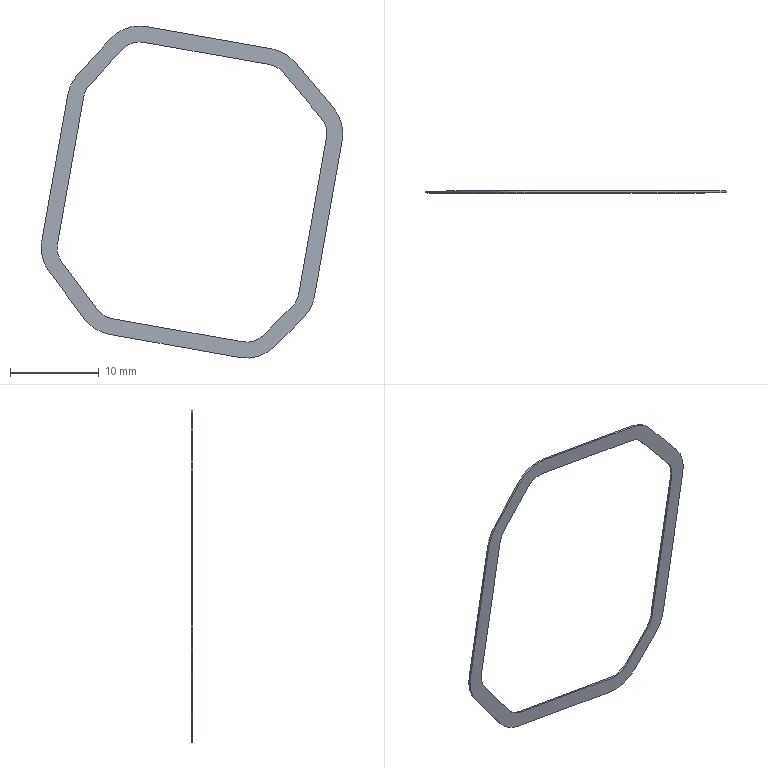Part | SolidWorks | features BaseBody 1 | 1 solid | 34 faces | box 34.044 x 0.2 x 37.494 mm | volume 39.583 mm3 | plane 18 | cylinder 16 | commonest cylinder face diameters 5.4 x8 9 x8
STEP:
#1=CARTESIAN_POINT('',(2064.15,-43.955,814.22));
#2=VERTEX_POINT('',#1);
#3=CARTESIAN_POINT('',(2064.15,-44.155,814.22));
#4=VERTEX_POINT('',#3);
#5=CARTESIAN_POINT('',(2064.15,-43.955,814.22));
#6=DIRECTION('',(0.,-1.,0.));
#7=VECTOR('',#6,1000.);
#8=LINE('',#5,#7);
#9=EDGE_CURVE('',#2,#4,#8,.T.);
#10=ORIENTED_EDGE('',*,*,#9,.T.);
#11=CARTESIAN_POINT('',(2049.484,-44.155,816.823));
#12=VERTEX_POINT('',#11);
#13=CARTESIAN_POINT('',(2049.484,-44.155,816.823));
#14=DIRECTION('',(0.9846,0.,-0.1747));
#15=VECTOR('',#14,1000.);
#16=LINE('',#13,#15);
#17=EDGE_CURVE('',#12,#4,#16,.T.);
#18=ORIENTED_EDGE('',*,*,#17,.F.);
#19=CARTESIAN_POINT('',(2049.484,-43.955,816.823));
#20=VERTEX_POINT('',#19);
#21=CARTESIAN_POINT('',(2049.484,-43.955,816.823));
#22=DIRECTION('',(0.,-1.,0.));
#23=VECTOR('',#22,1000.);
#24=LINE('',#21,#23);
#25=EDGE_CURVE('',#20,#12,#24,.T.);
#26=ORIENTED_EDGE('',*,*,#25,.F.);
#27=CARTESIAN_POINT('',(2049.484,-43.955,816.823));
#28=DIRECTION('',(0.9846,0.,-0.1747));
#29=VECTOR('',#28,1000.);
#30=LINE('',#27,#29);
#31=EDGE_CURVE('',#20,#2,#30,.T.);
#32=ORIENTED_EDGE('',*,*,#31,.T.);
#33=EDGE_LOOP('',(#10,#18,#26,#32));
#34=FACE_OUTER_BOUND('',#33,.T.);
#35=CARTESIAN_POINT('',(2049.484,-43.955,816.823));
#36=DIRECTION('',(-0.1747,0.,-0.9846));
#37=DIRECTION('',(-0.9846,0.,0.1747));
#38=AXIS2_PLACEMENT_3D('',#35,#36,#37);
#39=PLANE('',#38);
#40=ADVANCED_FACE('',(#34),#39,.T.);
#41=ORIENTED_EDGE('',*,*,#31,.F.);
#42=CARTESIAN_POINT('',(2046.674,-43.955,818.55));
#43=VERTEX_POINT('',#42);
#44=CARTESIAN_POINT('',(2050.27,-43.955,821.254));
#45=DIRECTION('',(0.,-1.,0.));
#46=DIRECTION('',(-0.7993,0.,-0.6009));
#47=AXIS2_PLACEMENT_3D('',#44,#45,#46);
#48=CIRCLE('',#47,4.5);
#49=EDGE_CURVE('',#43,#20,#48,.T.);
#50=ORIENTED_EDGE('',*,*,#49,.F.);
#51=CARTESIAN_POINT('',(2042.664,-43.955,823.882));
#52=VERTEX_POINT('',#51);
#53=CARTESIAN_POINT('',(2042.664,-43.955,823.882));
#54=DIRECTION('',(0.6009,0.,-0.7993));
#55=VECTOR('',#54,1000.);
#56=LINE('',#53,#55);
#57=EDGE_CURVE('',#52,#43,#56,.T.);
#58=ORIENTED_EDGE('',*,*,#57,.F.);
#59=CARTESIAN_POINT('',(2041.831,-43.955,827.373));
#60=VERTEX_POINT('',#59);
#61=CARTESIAN_POINT('',(2046.261,-43.955,826.586));
#62=DIRECTION('',(0.,-1.,0.));
#63=DIRECTION('',(-0.9846,0.,0.1747));
#64=AXIS2_PLACEMENT_3D('',#61,#62,#63);
#65=CIRCLE('',#64,4.5);
#66=EDGE_CURVE('',#60,#52,#65,.T.);
#67=ORIENTED_EDGE('',*,*,#66,.F.);
#68=CARTESIAN_POINT('',(2044.766,-43.955,843.914));
#69=VERTEX_POINT('',#68);
#70=CARTESIAN_POINT('',(2044.766,-43.955,843.914));
#71=DIRECTION('',(-0.1747,0.,-0.9846));
#72=VECTOR('',#71,1000.);
#73=LINE('',#70,#72);
#74=EDGE_CURVE('',#69,#60,#73,.T.);
#75=ORIENTED_EDGE('',*,*,#74,.F.);
#76=CARTESIAN_POINT('',(2045.883,-43.955,846.172));
#77=VERTEX_POINT('',#76);
#78=CARTESIAN_POINT('',(2049.197,-43.955,843.128));
#79=DIRECTION('',(0.,-1.,0.));
#80=DIRECTION('',(-0.7365,0.,0.6764));
#81=AXIS2_PLACEMENT_3D('',#78,#79,#80);
#82=CIRCLE('',#81,4.5);
#83=EDGE_CURVE('',#77,#69,#82,.T.);
#84=ORIENTED_EDGE('',*,*,#83,.F.);
#85=CARTESIAN_POINT('',(2049.572,-43.955,850.189));
#86=VERTEX_POINT('',#85);
#87=CARTESIAN_POINT('',(2049.572,-43.955,850.189));
#88=DIRECTION('',(-0.6764,0.,-0.7365));
#89=VECTOR('',#88,1000.);
#90=LINE('',#87,#89);
#91=EDGE_CURVE('',#86,#77,#90,.T.);
#92=ORIENTED_EDGE('',*,*,#91,.F.);
#93=CARTESIAN_POINT('',(2053.673,-43.955,851.576));
#94=VERTEX_POINT('',#93);
#95=CARTESIAN_POINT('',(2052.886,-43.955,847.145));
#96=DIRECTION('',(0.,-1.,0.));
#97=DIRECTION('',(0.1747,0.,0.9846));
#98=AXIS2_PLACEMENT_3D('',#95,#96,#97);
#99=CIRCLE('',#98,4.5);
#100=EDGE_CURVE('',#94,#86,#99,.T.);
#101=ORIENTED_EDGE('',*,*,#100,.F.);
#102=CARTESIAN_POINT('',(2067.797,-43.955,849.069));
#103=VERTEX_POINT('',#102);
#104=CARTESIAN_POINT('',(2067.797,-43.955,849.069));
#105=DIRECTION('',(-0.9846,0.,0.1747));
#106=VECTOR('',#105,1000.);
#107=LINE('',#104,#106);
#108=EDGE_CURVE('',#103,#94,#107,.T.);
#109=ORIENTED_EDGE('',*,*,#108,.F.);
#110=CARTESIAN_POINT('',(2070.461,-43.955,847.527));
#111=VERTEX_POINT('',#110);
#112=CARTESIAN_POINT('',(2067.011,-43.955,844.638));
#113=DIRECTION('',(0.,-1.,0.));
#114=DIRECTION('',(0.7668,0.,0.6419));
#115=AXIS2_PLACEMENT_3D('',#112,#113,#114);
#116=CIRCLE('',#115,4.5);
#117=EDGE_CURVE('',#111,#103,#116,.T.);
#118=ORIENTED_EDGE('',*,*,#117,.F.);
#119=CARTESIAN_POINT('',(2074.755,-43.955,842.398));
#120=VERTEX_POINT('',#119);
#121=CARTESIAN_POINT('',(2074.755,-43.955,842.398));
#122=DIRECTION('',(-0.6419,0.,0.7668));
#123=VECTOR('',#122,1000.);
#124=LINE('',#121,#123);
#125=EDGE_CURVE('',#120,#111,#124,.T.);
#126=ORIENTED_EDGE('',*,*,#125,.F.);
#127=CARTESIAN_POINT('',(2075.736,-43.955,838.723));
#128=VERTEX_POINT('',#127);
#129=CARTESIAN_POINT('',(2071.305,-43.955,839.509));
#130=DIRECTION('',(0.,-1.,0.));
#131=DIRECTION('',(0.9846,0.,-0.1747));
#132=AXIS2_PLACEMENT_3D('',#129,#130,#131);
#133=CIRCLE('',#132,4.5);
#134=EDGE_CURVE('',#128,#120,#133,.T.);
#135=ORIENTED_EDGE('',*,*,#134,.F.);
#136=CARTESIAN_POINT('',(2072.608,-43.955,821.098));
#137=VERTEX_POINT('',#136);
#138=CARTESIAN_POINT('',(2072.608,-43.955,821.098));
#139=DIRECTION('',(0.1747,0.,0.9846));
#140=VECTOR('',#139,1000.);
#141=LINE('',#138,#140);
#142=EDGE_CURVE('',#137,#128,#141,.T.);
#143=ORIENTED_EDGE('',*,*,#142,.F.);
#144=CARTESIAN_POINT('',(2071.355,-43.955,818.699));
#145=VERTEX_POINT('',#144);
#146=CARTESIAN_POINT('',(2068.177,-43.955,821.884));
#147=DIRECTION('',(0.,-1.,0.));
#148=DIRECTION('',(0.7063,0.,-0.7079));
#149=AXIS2_PLACEMENT_3D('',#146,#147,#148);
#150=CIRCLE('',#149,4.5);
#151=EDGE_CURVE('',#145,#137,#150,.T.);
#152=ORIENTED_EDGE('',*,*,#151,.F.);
#153=CARTESIAN_POINT('',(2068.115,-43.955,815.465));
#154=VERTEX_POINT('',#153);
#155=CARTESIAN_POINT('',(2068.115,-43.955,815.465));
#156=DIRECTION('',(0.7079,0.,0.7063));
#157=VECTOR('',#156,1000.);
#158=LINE('',#155,#157);
#159=EDGE_CURVE('',#154,#145,#158,.T.);
#160=ORIENTED_EDGE('',*,*,#159,.F.);
#161=CARTESIAN_POINT('',(2064.936,-43.955,818.651));
#162=DIRECTION('',(0.,-1.,0.));
#163=DIRECTION('',(-0.1747,0.,-0.9846));
#164=AXIS2_PLACEMENT_3D('',#161,#162,#163);
#165=CIRCLE('',#164,4.5);
#166=EDGE_CURVE('',#2,#154,#165,.T.);
#167=ORIENTED_EDGE('',*,*,#166,.F.);
#168=EDGE_LOOP('',(#41,#50,#58,#67,#75,#84,#92,#101,#109,#118,#126,#135,#143,#152,#160,#167));
#169=FACE_OUTER_BOUND('',#168,.T.);
#170=CARTESIAN_POINT('',(2066.843,-43.955,816.74));
#171=VERTEX_POINT('',#170);
#172=CARTESIAN_POINT('',(2064.464,-43.955,815.992));
#173=VERTEX_POINT('',#172);
#174=CARTESIAN_POINT('',(2064.936,-43.955,818.651));
#175=DIRECTION('',(0.,1.,0.));
#176=DIRECTION('',(0.7063,0.,-0.7079));
#177=AXIS2_PLACEMENT_3D('',#174,#175,#176);
#178=CIRCLE('',#177,2.7);
#179=EDGE_CURVE('',#171,#173,#178,.T.);
#180=ORIENTED_EDGE('',*,*,#179,.F.);
#181=CARTESIAN_POINT('',(2070.084,-43.955,819.973));
#182=VERTEX_POINT('',#181);
#183=CARTESIAN_POINT('',(2070.084,-43.955,819.973));
#184=DIRECTION('',(-0.7079,0.,-0.7063));
#185=VECTOR('',#184,1000.);
#186=LINE('',#183,#185);
#187=EDGE_CURVE('',#182,#171,#186,.T.);
#188=ORIENTED_EDGE('',*,*,#187,.F.);
#189=CARTESIAN_POINT('',(2070.835,-43.955,821.413));
#190=VERTEX_POINT('',#189);
#191=CARTESIAN_POINT('',(2068.177,-43.955,821.884));
#192=DIRECTION('',(0.,1.,0.));
#193=DIRECTION('',(0.9846,0.,-0.1747));
#194=AXIS2_PLACEMENT_3D('',#191,#192,#193);
#195=CIRCLE('',#194,2.7);
#196=EDGE_CURVE('',#190,#182,#195,.T.);
#197=ORIENTED_EDGE('',*,*,#196,.F.);
#198=CARTESIAN_POINT('',(2073.963,-43.955,839.037));
#199=VERTEX_POINT('',#198);
#200=CARTESIAN_POINT('',(2073.963,-43.955,839.037));
#201=DIRECTION('',(-0.1747,0.,-0.9846));
#202=VECTOR('',#201,1000.);
#203=LINE('',#200,#202);
#204=EDGE_CURVE('',#199,#190,#203,.T.);
#205=ORIENTED_EDGE('',*,*,#204,.F.);
#206=CARTESIAN_POINT('',(2073.375,-43.955,841.242));
#207=VERTEX_POINT('',#206);
#208=CARTESIAN_POINT('',(2071.305,-43.955,839.509));
#209=DIRECTION('',(0.,1.,0.));
#210=DIRECTION('',(0.7668,0.,0.6419));
#211=AXIS2_PLACEMENT_3D('',#208,#209,#210);
#212=CIRCLE('',#211,2.7);
#213=EDGE_CURVE('',#207,#199,#212,.T.);
#214=ORIENTED_EDGE('',*,*,#213,.F.);
#215=CARTESIAN_POINT('',(2069.081,-43.955,846.371));
#216=VERTEX_POINT('',#215);
#217=CARTESIAN_POINT('',(2069.081,-43.955,846.371));
#218=DIRECTION('',(0.6419,0.,-0.7668));
#219=VECTOR('',#218,1000.);
#220=LINE('',#217,#219);
#221=EDGE_CURVE('',#216,#207,#220,.T.);
#222=ORIENTED_EDGE('',*,*,#221,.F.);
#223=CARTESIAN_POINT('',(2067.482,-43.955,847.297));
#224=VERTEX_POINT('',#223);
#225=CARTESIAN_POINT('',(2067.011,-43.955,844.638));
#226=DIRECTION('',(0.,1.,0.));
#227=DIRECTION('',(0.1747,0.,0.9846));
#228=AXIS2_PLACEMENT_3D('',#225,#226,#227);
#229=CIRCLE('',#228,2.7);
#230=EDGE_CURVE('',#224,#216,#229,.T.);
#231=ORIENTED_EDGE('',*,*,#230,.F.);
#232=CARTESIAN_POINT('',(2053.358,-43.955,849.803));
#233=VERTEX_POINT('',#232);
#234=CARTESIAN_POINT('',(2053.358,-43.955,849.803));
#235=DIRECTION('',(0.9846,0.,-0.1747));
#236=VECTOR('',#235,1000.);
#237=LINE('',#234,#236);
#238=EDGE_CURVE('',#233,#224,#237,.T.);
#239=ORIENTED_EDGE('',*,*,#238,.F.);
#240=CARTESIAN_POINT('',(2050.898,-43.955,848.971));
#241=VERTEX_POINT('',#240);
#242=CARTESIAN_POINT('',(2052.886,-43.955,847.145));
#243=DIRECTION('',(0.,1.,0.));
#244=DIRECTION('',(-0.7365,0.,0.6764));
#245=AXIS2_PLACEMENT_3D('',#242,#243,#244);
#246=CIRCLE('',#245,2.7);
#247=EDGE_CURVE('',#241,#233,#246,.T.);
#248=ORIENTED_EDGE('',*,*,#247,.F.);
#249=CARTESIAN_POINT('',(2047.209,-43.955,844.954));
#250=VERTEX_POINT('',#249);
#251=CARTESIAN_POINT('',(2047.209,-43.955,844.954));
#252=DIRECTION('',(0.6764,0.,0.7365));
#253=VECTOR('',#252,1000.);
#254=LINE('',#251,#253);
#255=EDGE_CURVE('',#250,#241,#254,.T.);
#256=ORIENTED_EDGE('',*,*,#255,.F.);
#257=CARTESIAN_POINT('',(2046.539,-43.955,843.6));
#258=VERTEX_POINT('',#257);
#259=CARTESIAN_POINT('',(2049.197,-43.955,843.128));
#260=DIRECTION('',(0.,1.,0.));
#261=DIRECTION('',(-0.9846,0.,0.1747));
#262=AXIS2_PLACEMENT_3D('',#259,#260,#261);
#263=CIRCLE('',#262,2.7);
#264=EDGE_CURVE('',#258,#250,#263,.T.);
#265=ORIENTED_EDGE('',*,*,#264,.F.);
#266=CARTESIAN_POINT('',(2043.603,-43.955,827.058));
#267=VERTEX_POINT('',#266);
#268=CARTESIAN_POINT('',(2043.603,-43.955,827.058));
#269=DIRECTION('',(0.1747,0.,0.9846));
#270=VECTOR('',#269,1000.);
#271=LINE('',#268,#270);
#272=EDGE_CURVE('',#267,#258,#271,.T.);
#273=ORIENTED_EDGE('',*,*,#272,.F.);
#274=CARTESIAN_POINT('',(2044.103,-43.955,824.964));
#275=VERTEX_POINT('',#274);
#276=CARTESIAN_POINT('',(2046.261,-43.955,826.586));
#277=DIRECTION('',(0.,1.,0.));
#278=DIRECTION('',(-0.7993,0.,-0.6009));
#279=AXIS2_PLACEMENT_3D('',#276,#277,#278);
#280=CIRCLE('',#279,2.7);
#281=EDGE_CURVE('',#275,#267,#280,.T.);
#282=ORIENTED_EDGE('',*,*,#281,.F.);
#283=CARTESIAN_POINT('',(2048.112,-43.955,819.631));
#284=VERTEX_POINT('',#283);
#285=CARTESIAN_POINT('',(2048.112,-43.955,819.631));
#286=DIRECTION('',(-0.6009,0.,0.7993));
#287=VECTOR('',#286,1000.);
#288=LINE('',#285,#287);
#289=EDGE_CURVE('',#284,#275,#288,.T.);
#290=ORIENTED_EDGE('',*,*,#289,.F.);
#291=CARTESIAN_POINT('',(2049.799,-43.955,818.595));
#292=VERTEX_POINT('',#291);
#293=CARTESIAN_POINT('',(2050.27,-43.955,821.254));
#294=DIRECTION('',(0.,1.,0.));
#295=DIRECTION('',(-0.1747,0.,-0.9846));
#296=AXIS2_PLACEMENT_3D('',#293,#294,#295);
#297=CIRCLE('',#296,2.7);
#298=EDGE_CURVE('',#292,#284,#297,.T.);
#299=ORIENTED_EDGE('',*,*,#298,.F.);
#300=CARTESIAN_POINT('',(2064.464,-43.955,815.992));
#301=DIRECTION('',(-0.9846,0.,0.1747));
#302=VECTOR('',#301,1000.);
#303=LINE('',#300,#302);
#304=EDGE_CURVE('',#173,#292,#303,.T.);
#305=ORIENTED_EDGE('',*,*,#304,.F.);
#306=EDGE_LOOP('',(#180,#188,#197,#205,#214,#222,#231,#239,#248,#256,#265,#273,#282,#290,#299,#305));
#307=FACE_BOUND('',#306,.T.);
#308=CARTESIAN_POINT('',(2032.4,-43.955,838.898));
#309=DIRECTION('',(0.,-1.,0.));
#310=DIRECTION('',(-0.9846,0.,0.1747));
#311=AXIS2_PLACEMENT_3D('',#308,#309,#310);
#312=PLANE('',#311);
#313=ADVANCED_FACE('',(#169,#307),#312,.F.);
#314=CARTESIAN_POINT('',(2068.115,-44.155,815.465));
#315=VERTEX_POINT('',#314);
#316=CARTESIAN_POINT('',(2068.115,-43.955,815.465));
#317=DIRECTION('',(0.,-1.,0.));
#318=VECTOR('',#317,1000.);
#319=LINE('',#316,#318);
#320=EDGE_CURVE('',#154,#315,#319,.T.);
#321=ORIENTED_EDGE('',*,*,#320,.T.);
#322=CARTESIAN_POINT('',(2064.936,-44.155,818.651));
#323=DIRECTION('',(0.,-1.,0.));
#324=DIRECTION('',(-0.1747,0.,-0.9846));
#325=AXIS2_PLACEMENT_3D('',#322,#323,#324);
#326=CIRCLE('',#325,4.5);
#327=EDGE_CURVE('',#4,#315,#326,.T.);
#328=ORIENTED_EDGE('',*,*,#327,.F.);
#329=ORIENTED_EDGE('',*,*,#9,.F.);
#330=ORIENTED_EDGE('',*,*,#166,.T.);
#331=EDGE_LOOP('',(#321,#328,#329,#330));
#332=FACE_OUTER_BOUND('',#331,.T.);
#333=CARTESIAN_POINT('',(2064.936,-43.955,818.651));
#334=DIRECTION('',(0.,-1.,0.));
#335=DIRECTION('',(-0.9846,0.,0.1747));
#336=AXIS2_PLACEMENT_3D('',#333,#334,#335);
#337=CYLINDRICAL_SURFACE('',#336,4.5);
#338=ADVANCED_FACE('',(#332),#337,.T.);
#339=CARTESIAN_POINT('',(2071.355,-44.155,818.699));
#340=VERTEX_POINT('',#339);
#341=CARTESIAN_POINT('',(2068.115,-44.155,815.465));
#342=DIRECTION('',(0.7079,0.,0.7063));
#343=VECTOR('',#342,1000.);
#344=LINE('',#341,#343);
#345=EDGE_CURVE('',#315,#340,#344,.T.);
#346=ORIENTED_EDGE('',*,*,#345,.T.);
#347=CARTESIAN_POINT('',(2072.608,-44.155,821.098));
#348=VERTEX_POINT('',#347);
#349=CARTESIAN_POINT('',(2068.177,-44.155,821.884));
#350=DIRECTION('',(0.,-1.,0.));
#351=DIRECTION('',(0.7063,0.,-0.7079));
#352=AXIS2_PLACEMENT_3D('',#349,#350,#351);
#353=CIRCLE('',#352,4.5);
#354=EDGE_CURVE('',#340,#348,#353,.T.);
#355=ORIENTED_EDGE('',*,*,#354,.T.);
#356=CARTESIAN_POINT('',(2075.736,-44.155,838.723));
#357=VERTEX_POINT('',#356);
#358=CARTESIAN_POINT('',(2072.608,-44.155,821.098));
#359=DIRECTION('',(0.1747,0.,0.9846));
#360=VECTOR('',#359,1000.);
#361=LINE('',#358,#360);
#362=EDGE_CURVE('',#348,#357,#361,.T.);
#363=ORIENTED_EDGE('',*,*,#362,.T.);
#364=CARTESIAN_POINT('',(2074.755,-44.155,842.398));
#365=VERTEX_POINT('',#364);
#366=CARTESIAN_POINT('',(2071.305,-44.155,839.509));
#367=DIRECTION('',(0.,-1.,0.));
#368=DIRECTION('',(0.9846,0.,-0.1747));
#369=AXIS2_PLACEMENT_3D('',#366,#367,#368);
#370=CIRCLE('',#369,4.5);
#371=EDGE_CURVE('',#357,#365,#370,.T.);
#372=ORIENTED_EDGE('',*,*,#371,.T.);
#373=CARTESIAN_POINT('',(2070.461,-44.155,847.527));
#374=VERTEX_POINT('',#373);
#375=CARTESIAN_POINT('',(2074.755,-44.155,842.398));
#376=DIRECTION('',(-0.6419,0.,0.7668));
#377=VECTOR('',#376,1000.);
#378=LINE('',#375,#377);
#379=EDGE_CURVE('',#365,#374,#378,.T.);
#380=ORIENTED_EDGE('',*,*,#379,.T.);
#381=CARTESIAN_POINT('',(2067.797,-44.155,849.069));
#382=VERTEX_POINT('',#381);
#383=CARTESIAN_POINT('',(2067.011,-44.155,844.638));
#384=DIRECTION('',(0.,-1.,0.));
#385=DIRECTION('',(0.7668,0.,0.6419));
#386=AXIS2_PLACEMENT_3D('',#383,#384,#385);
#387=CIRCLE('',#386,4.5);
#388=EDGE_CURVE('',#374,#382,#387,.T.);
#389=ORIENTED_EDGE('',*,*,#388,.T.);
#390=CARTESIAN_POINT('',(2053.673,-44.155,851.576));
#391=VERTEX_POINT('',#390);
#392=CARTESIAN_POINT('',(2067.797,-44.155,849.069));
#393=DIRECTION('',(-0.9846,0.,0.1747));
#394=VECTOR('',#393,1000.);
#395=LINE('',#392,#394);
#396=EDGE_CURVE('',#382,#391,#395,.T.);
#397=ORIENTED_EDGE('',*,*,#396,.T.);
#398=CARTESIAN_POINT('',(2049.572,-44.155,850.189));
#399=VERTEX_POINT('',#398);
#400=CARTESIAN_POINT('',(2052.886,-44.155,847.145));
#401=DIRECTION('',(0.,-1.,0.));
#402=DIRECTION('',(0.1747,0.,0.9846));
#403=AXIS2_PLACEMENT_3D('',#400,#401,#402);
#404=CIRCLE('',#403,4.5);
#405=EDGE_CURVE('',#391,#399,#404,.T.);
#406=ORIENTED_EDGE('',*,*,#405,.T.);
#407=CARTESIAN_POINT('',(2045.883,-44.155,846.172));
#408=VERTEX_POINT('',#407);
#409=CARTESIAN_POINT('',(2049.572,-44.155,850.189));
#410=DIRECTION('',(-0.6764,0.,-0.7365));
#411=VECTOR('',#410,1000.);
#412=LINE('',#409,#411);
#413=EDGE_CURVE('',#399,#408,#412,.T.);
#414=ORIENTED_EDGE('',*,*,#413,.T.);
#415=CARTESIAN_POINT('',(2044.766,-44.155,843.914));
#416=VERTEX_POINT('',#415);
#417=CARTESIAN_POINT('',(2049.197,-44.155,843.128));
#418=DIRECTION('',(0.,-1.,0.));
#419=DIRECTION('',(-0.7365,0.,0.6764));
#420=AXIS2_PLACEMENT_3D('',#417,#418,#419);
#421=CIRCLE('',#420,4.5);
#422=EDGE_CURVE('',#408,#416,#421,.T.);
#423=ORIENTED_EDGE('',*,*,#422,.T.);
#424=CARTESIAN_POINT('',(2041.831,-44.155,827.373));
#425=VERTEX_POINT('',#424);
#426=CARTESIAN_POINT('',(2044.766,-44.155,843.914));
#427=DIRECTION('',(-0.1747,0.,-0.9846));
#428=VECTOR('',#427,1000.);
#429=LINE('',#426,#428);
#430=EDGE_CURVE('',#416,#425,#429,.T.);
#431=ORIENTED_EDGE('',*,*,#430,.T.);
#432=CARTESIAN_POINT('',(2042.664,-44.155,823.882));
#433=VERTEX_POINT('',#432);
#434=CARTESIAN_POINT('',(2046.261,-44.155,826.586));
#435=DIRECTION('',(0.,-1.,0.));
#436=DIRECTION('',(-0.9846,0.,0.1747));
#437=AXIS2_PLACEMENT_3D('',#434,#435,#436);
#438=CIRCLE('',#437,4.5);
#439=EDGE_CURVE('',#425,#433,#438,.T.);
#440=ORIENTED_EDGE('',*,*,#439,.T.);
#441=CARTESIAN_POINT('',(2046.674,-44.155,818.55));
#442=VERTEX_POINT('',#441);
#443=CARTESIAN_POINT('',(2042.664,-44.155,823.882));
#444=DIRECTION('',(0.6009,0.,-0.7993));
#445=VECTOR('',#444,1000.);
#446=LINE('',#443,#445);
#447=EDGE_CURVE('',#433,#442,#446,.T.);
#448=ORIENTED_EDGE('',*,*,#447,.T.);
#449=CARTESIAN_POINT('',(2050.27,-44.155,821.254));
#450=DIRECTION('',(0.,-1.,0.));
#451=DIRECTION('',(-0.7993,0.,-0.6009));
#452=AXIS2_PLACEMENT_3D('',#449,#450,#451);
#453=CIRCLE('',#452,4.5);
#454=EDGE_CURVE('',#442,#12,#453,.T.);
#455=ORIENTED_EDGE('',*,*,#454,.T.);
#456=ORIENTED_EDGE('',*,*,#17,.T.);
#457=ORIENTED_EDGE('',*,*,#327,.T.);
#458=EDGE_LOOP('',(#346,#355,#363,#372,#380,#389,#397,#406,#414,#423,#431,#440,#448,#455,#456,#457));
#459=FACE_OUTER_BOUND('',#458,.T.);
#460=CARTESIAN_POINT('',(2049.799,-44.155,818.595));
#461=VERTEX_POINT('',#460);
#462=CARTESIAN_POINT('',(2048.112,-44.155,819.631));
#463=VERTEX_POINT('',#462);
#464=CARTESIAN_POINT('',(2050.27,-44.155,821.254));
#465=DIRECTION('',(0.,1.,0.));
#466=DIRECTION('',(-0.1747,0.,-0.9846));
#467=AXIS2_PLACEMENT_3D('',#464,#465,#466);
#468=CIRCLE('',#467,2.7);
#469=EDGE_CURVE('',#461,#463,#468,.T.);
#470=ORIENTED_EDGE('',*,*,#469,.T.);
#471=CARTESIAN_POINT('',(2044.103,-44.155,824.964));
#472=VERTEX_POINT('',#471);
#473=CARTESIAN_POINT('',(2048.112,-44.155,819.631));
#474=DIRECTION('',(-0.6009,0.,0.7993));
#475=VECTOR('',#474,1000.);
#476=LINE('',#473,#475);
#477=EDGE_CURVE('',#463,#472,#476,.T.);
#478=ORIENTED_EDGE('',*,*,#477,.T.);
#479=CARTESIAN_POINT('',(2043.603,-44.155,827.058));
#480=VERTEX_POINT('',#479);
#481=CARTESIAN_POINT('',(2046.261,-44.155,826.586));
#482=DIRECTION('',(0.,1.,0.));
#483=DIRECTION('',(-0.7993,0.,-0.6009));
#484=AXIS2_PLACEMENT_3D('',#481,#482,#483);
#485=CIRCLE('',#484,2.7);
#486=EDGE_CURVE('',#472,#480,#485,.T.);
#487=ORIENTED_EDGE('',*,*,#486,.T.);
#488=CARTESIAN_POINT('',(2046.539,-44.155,843.6));
#489=VERTEX_POINT('',#488);
#490=CARTESIAN_POINT('',(2043.603,-44.155,827.058));
#491=DIRECTION('',(0.1747,0.,0.9846));
#492=VECTOR('',#491,1000.);
#493=LINE('',#490,#492);
#494=EDGE_CURVE('',#480,#489,#493,.T.);
#495=ORIENTED_EDGE('',*,*,#494,.T.);
#496=CARTESIAN_POINT('',(2047.209,-44.155,844.954));
#497=VERTEX_POINT('',#496);
#498=CARTESIAN_POINT('',(2049.197,-44.155,843.128));
#499=DIRECTION('',(0.,1.,0.));
#500=DIRECTION('',(-0.9846,0.,0.1747));
#501=AXIS2_PLACEMENT_3D('',#498,#499,#500);
#502=CIRCLE('',#501,2.7);
#503=EDGE_CURVE('',#489,#497,#502,.T.);
#504=ORIENTED_EDGE('',*,*,#503,.T.);
#505=CARTESIAN_POINT('',(2050.898,-44.155,848.971));
#506=VERTEX_POINT('',#505);
#507=CARTESIAN_POINT('',(2047.209,-44.155,844.954));
#508=DIRECTION('',(0.6764,0.,0.7365));
#509=VECTOR('',#508,1000.);
#510=LINE('',#507,#509);
#511=EDGE_CURVE('',#497,#506,#510,.T.);
#512=ORIENTED_EDGE('',*,*,#511,.T.);
#513=CARTESIAN_POINT('',(2053.358,-44.155,849.803));
#514=VERTEX_POINT('',#513);
#515=CARTESIAN_POINT('',(2052.886,-44.155,847.145));
#516=DIRECTION('',(0.,1.,0.));
#517=DIRECTION('',(-0.7365,0.,0.6764));
#518=AXIS2_PLACEMENT_3D('',#515,#516,#517);
#519=CIRCLE('',#518,2.7);
#520=EDGE_CURVE('',#506,#514,#519,.T.);
#521=ORIENTED_EDGE('',*,*,#520,.T.);
#522=CARTESIAN_POINT('',(2067.482,-44.155,847.297));
#523=VERTEX_POINT('',#522);
#524=CARTESIAN_POINT('',(2053.358,-44.155,849.803));
#525=DIRECTION('',(0.9846,0.,-0.1747));
#526=VECTOR('',#525,1000.);
#527=LINE('',#524,#526);
#528=EDGE_CURVE('',#514,#523,#527,.T.);
#529=ORIENTED_EDGE('',*,*,#528,.T.);
#530=CARTESIAN_POINT('',(2069.081,-44.155,846.371));
#531=VERTEX_POINT('',#530);
#532=CARTESIAN_POINT('',(2067.011,-44.155,844.638));
#533=DIRECTION('',(0.,1.,0.));
#534=DIRECTION('',(0.1747,0.,0.9846));
#535=AXIS2_PLACEMENT_3D('',#532,#533,#534);
#536=CIRCLE('',#535,2.7);
#537=EDGE_CURVE('',#523,#531,#536,.T.);
#538=ORIENTED_EDGE('',*,*,#537,.T.);
#539=CARTESIAN_POINT('',(2073.375,-44.155,841.242));
#540=VERTEX_POINT('',#539);
#541=CARTESIAN_POINT('',(2069.081,-44.155,846.371));
#542=DIRECTION('',(0.6419,0.,-0.7668));
#543=VECTOR('',#542,1000.);
#544=LINE('',#541,#543);
#545=EDGE_CURVE('',#531,#540,#544,.T.);
#546=ORIENTED_EDGE('',*,*,#545,.T.);
#547=CARTESIAN_POINT('',(2073.963,-44.155,839.037));
#548=VERTEX_POINT('',#547);
#549=CARTESIAN_POINT('',(2071.305,-44.155,839.509));
#550=DIRECTION('',(0.,1.,0.));
#551=DIRECTION('',(0.7668,0.,0.6419));
#552=AXIS2_PLACEMENT_3D('',#549,#550,#551);
#553=CIRCLE('',#552,2.7);
#554=EDGE_CURVE('',#540,#548,#553,.T.);
#555=ORIENTED_EDGE('',*,*,#554,.T.);
#556=CARTESIAN_POINT('',(2070.835,-44.155,821.413));
#557=VERTEX_POINT('',#556);
#558=CARTESIAN_POINT('',(2073.963,-44.155,839.037));
#559=DIRECTION('',(-0.1747,0.,-0.9846));
#560=VECTOR('',#559,1000.);
#561=LINE('',#558,#560);
#562=EDGE_CURVE('',#548,#557,#561,.T.);
#563=ORIENTED_EDGE('',*,*,#562,.T.);
#564=CARTESIAN_POINT('',(2070.084,-44.155,819.973));
#565=VERTEX_POINT('',#564);
#566=CARTESIAN_POINT('',(2068.177,-44.155,821.884));
#567=DIRECTION('',(0.,1.,0.));
#568=DIRECTION('',(0.9846,0.,-0.1747));
#569=AXIS2_PLACEMENT_3D('',#566,#567,#568);
#570=CIRCLE('',#569,2.7);
#571=EDGE_CURVE('',#557,#565,#570,.T.);
#572=ORIENTED_EDGE('',*,*,#571,.T.);
#573=CARTESIAN_POINT('',(2066.843,-44.155,816.74));
#574=VERTEX_POINT('',#573);
#575=CARTESIAN_POINT('',(2070.084,-44.155,819.973));
#576=DIRECTION('',(-0.7079,0.,-0.7063));
#577=VECTOR('',#576,1000.);
#578=LINE('',#575,#577);
#579=EDGE_CURVE('',#565,#574,#578,.T.);
#580=ORIENTED_EDGE('',*,*,#579,.T.);
#581=CARTESIAN_POINT('',(2064.464,-44.155,815.992));
#582=VERTEX_POINT('',#581);
#583=CARTESIAN_POINT('',(2064.936,-44.155,818.651));
#584=DIRECTION('',(0.,1.,0.));
#585=DIRECTION('',(0.7063,0.,-0.7079));
#586=AXIS2_PLACEMENT_3D('',#583,#584,#585);
#587=CIRCLE('',#586,2.7);
#588=EDGE_CURVE('',#574,#582,#587,.T.);
#589=ORIENTED_EDGE('',*,*,#588,.T.);
#590=CARTESIAN_POINT('',(2064.464,-44.155,815.992));
#591=DIRECTION('',(-0.9846,0.,0.1747));
#592=VECTOR('',#591,1000.);
#593=LINE('',#590,#592);
#594=EDGE_CURVE('',#582,#461,#593,.T.);
#595=ORIENTED_EDGE('',*,*,#594,.T.);
#596=EDGE_LOOP('',(#470,#478,#487,#495,#504,#512,#521,#529,#538,#546,#555,#563,#572,#580,#589,#595));
#597=FACE_BOUND('',#596,.T.);
#598=CARTESIAN_POINT('',(2032.4,-44.155,838.898));
#599=DIRECTION('',(0.,-1.,0.));
#600=DIRECTION('',(-0.9846,0.,0.1747));
#601=AXIS2_PLACEMENT_3D('',#598,#599,#600);
#602=PLANE('',#601);
#603=ADVANCED_FACE('',(#459,#597),#602,.T.);
#604=ORIENTED_EDGE('',*,*,#25,.T.);
#605=ORIENTED_EDGE('',*,*,#454,.F.);
#606=CARTESIAN_POINT('',(2046.674,-43.955,818.55));
#607=DIRECTION('',(0.,-1.,0.));
#608=VECTOR('',#607,1000.);
#609=LINE('',#606,#608);
#610=EDGE_CURVE('',#43,#442,#609,.T.);
#611=ORIENTED_EDGE('',*,*,#610,.F.);
#612=ORIENTED_EDGE('',*,*,#49,.T.);
#613=EDGE_LOOP('',(#604,#605,#611,#612));
#614=FACE_OUTER_BOUND('',#613,.T.);
#615=CARTESIAN_POINT('',(2050.27,-43.955,821.254));
#616=DIRECTION('',(0.,-1.,0.));
#617=DIRECTION('',(-0.9846,0.,0.1747));
#618=AXIS2_PLACEMENT_3D('',#615,#616,#617);
#619=CYLINDRICAL_SURFACE('',#618,4.5);
#620=ADVANCED_FACE('',(#614),#619,.T.);
#621=ORIENTED_EDGE('',*,*,#610,.T.);
#622=ORIENTED_EDGE('',*,*,#447,.F.);
#623=CARTESIAN_POINT('',(2042.664,-43.955,823.882));
#624=DIRECTION('',(0.,-1.,0.));
#625=VECTOR('',#624,1000.);
#626=LINE('',#623,#625);
#627=EDGE_CURVE('',#52,#433,#626,.T.);
#628=ORIENTED_EDGE('',*,*,#627,.F.);
#629=ORIENTED_EDGE('',*,*,#57,.T.);
#630=EDGE_LOOP('',(#621,#622,#628,#629));
#631=FACE_OUTER_BOUND('',#630,.T.);
#632=CARTESIAN_POINT('',(2042.664,-43.955,823.882));
#633=DIRECTION('',(-0.7993,0.,-0.6009));
#634=DIRECTION('',(-0.6009,0.,0.7993));
#635=AXIS2_PLACEMENT_3D('',#632,#633,#634);
#636=PLANE('',#635);
#637=ADVANCED_FACE('',(#631),#636,.T.);
#638=ORIENTED_EDGE('',*,*,#627,.T.);
#639=ORIENTED_EDGE('',*,*,#439,.F.);
#640=CARTESIAN_POINT('',(2041.831,-43.955,827.373));
#641=DIRECTION('',(0.,-1.,0.));
#642=VECTOR('',#641,1000.);
#643=LINE('',#640,#642);
#644=EDGE_CURVE('',#60,#425,#643,.T.);
#645=ORIENTED_EDGE('',*,*,#644,.F.);
#646=ORIENTED_EDGE('',*,*,#66,.T.);
#647=EDGE_LOOP('',(#638,#639,#645,#646));
#648=FACE_OUTER_BOUND('',#647,.T.);
#649=CARTESIAN_POINT('',(2046.261,-43.955,826.586));
#650=DIRECTION('',(0.,-1.,0.));
#651=DIRECTION('',(-0.9846,0.,0.1747));
#652=AXIS2_PLACEMENT_3D('',#649,#650,#651);
#653=CYLINDRICAL_SURFACE('',#652,4.5);
#654=ADVANCED_FACE('',(#648),#653,.T.);
#655=ORIENTED_EDGE('',*,*,#644,.T.);
#656=ORIENTED_EDGE('',*,*,#430,.F.);
#657=CARTESIAN_POINT('',(2044.766,-43.955,843.914));
#658=DIRECTION('',(0.,-1.,0.));
#659=VECTOR('',#658,1000.);
#660=LINE('',#657,#659);
#661=EDGE_CURVE('',#69,#416,#660,.T.);
#662=ORIENTED_EDGE('',*,*,#661,.F.);
#663=ORIENTED_EDGE('',*,*,#74,.T.);
#664=EDGE_LOOP('',(#655,#656,#662,#663));
#665=FACE_OUTER_BOUND('',#664,.T.);
#666=CARTESIAN_POINT('',(2044.766,-43.955,843.914));
#667=DIRECTION('',(-0.9846,0.,0.1747));
#668=DIRECTION('',(0.1747,0.,0.9846));
#669=AXIS2_PLACEMENT_3D('',#666,#667,#668);
#670=PLANE('',#669);
#671=ADVANCED_FACE('',(#665),#670,.T.);
#672=ORIENTED_EDGE('',*,*,#661,.T.);
#673=ORIENTED_EDGE('',*,*,#422,.F.);
#674=CARTESIAN_POINT('',(2045.883,-43.955,846.172));
#675=DIRECTION('',(0.,-1.,0.));
#676=VECTOR('',#675,1000.);
#677=LINE('',#674,#676);
#678=EDGE_CURVE('',#77,#408,#677,.T.);
#679=ORIENTED_EDGE('',*,*,#678,.F.);
#680=ORIENTED_EDGE('',*,*,#83,.T.);
#681=EDGE_LOOP('',(#672,#673,#679,#680));
#682=FACE_OUTER_BOUND('',#681,.T.);
#683=CARTESIAN_POINT('',(2049.197,-43.955,843.128));
#684=DIRECTION('',(0.,-1.,0.));
#685=DIRECTION('',(-0.9846,0.,0.1747));
#686=AXIS2_PLACEMENT_3D('',#683,#684,#685);
#687=CYLINDRICAL_SURFACE('',#686,4.5);
#688=ADVANCED_FACE('',(#682),#687,.T.);
#689=ORIENTED_EDGE('',*,*,#678,.T.);
#690=ORIENTED_EDGE('',*,*,#413,.F.);
#691=CARTESIAN_POINT('',(2049.572,-43.955,850.189));
#692=DIRECTION('',(0.,-1.,0.));
#693=VECTOR('',#692,1000.);
#694=LINE('',#691,#693);
#695=EDGE_CURVE('',#86,#399,#694,.T.);
#696=ORIENTED_EDGE('',*,*,#695,.F.);
#697=ORIENTED_EDGE('',*,*,#91,.T.);
#698=EDGE_LOOP('',(#689,#690,#696,#697));
#699=FACE_OUTER_BOUND('',#698,.T.);
#700=CARTESIAN_POINT('',(2049.572,-43.955,850.189));
#701=DIRECTION('',(-0.7365,0.,0.6764));
#702=DIRECTION('',(0.6764,0.,0.7365));
#703=AXIS2_PLACEMENT_3D('',#700,#701,#702);
#704=PLANE('',#703);
#705=ADVANCED_FACE('',(#699),#704,.T.);
#706=ORIENTED_EDGE('',*,*,#695,.T.);
#707=ORIENTED_EDGE('',*,*,#405,.F.);
#708=CARTESIAN_POINT('',(2053.673,-43.955,851.576));
#709=DIRECTION('',(0.,-1.,0.));
#710=VECTOR('',#709,1000.);
#711=LINE('',#708,#710);
#712=EDGE_CURVE('',#94,#391,#711,.T.);
#713=ORIENTED_EDGE('',*,*,#712,.F.);
#714=ORIENTED_EDGE('',*,*,#100,.T.);
#715=EDGE_LOOP('',(#706,#707,#713,#714));
#716=FACE_OUTER_BOUND('',#715,.T.);
#717=CARTESIAN_POINT('',(2052.886,-43.955,847.145));
#718=DIRECTION('',(0.,-1.,0.));
#719=DIRECTION('',(-0.9846,0.,0.1747));
#720=AXIS2_PLACEMENT_3D('',#717,#718,#719);
#721=CYLINDRICAL_SURFACE('',#720,4.5);
#722=ADVANCED_FACE('',(#716),#721,.T.);
#723=ORIENTED_EDGE('',*,*,#712,.T.);
#724=ORIENTED_EDGE('',*,*,#396,.F.);
#725=CARTESIAN_POINT('',(2067.797,-43.955,849.069));
#726=DIRECTION('',(0.,-1.,0.));
#727=VECTOR('',#726,1000.);
#728=LINE('',#725,#727);
#729=EDGE_CURVE('',#103,#382,#728,.T.);
#730=ORIENTED_EDGE('',*,*,#729,.F.);
#731=ORIENTED_EDGE('',*,*,#108,.T.);
#732=EDGE_LOOP('',(#723,#724,#730,#731));
#733=FACE_OUTER_BOUND('',#732,.T.);
#734=CARTESIAN_POINT('',(2067.797,-43.955,849.069));
#735=DIRECTION('',(0.1747,0.,0.9846));
#736=DIRECTION('',(0.9846,0.,-0.1747));
#737=AXIS2_PLACEMENT_3D('',#734,#735,#736);
#738=PLANE('',#737);
#739=ADVANCED_FACE('',(#733),#738,.T.);
#740=ORIENTED_EDGE('',*,*,#729,.T.);
#741=ORIENTED_EDGE('',*,*,#388,.F.);
#742=CARTESIAN_POINT('',(2070.461,-43.955,847.527));
#743=DIRECTION('',(0.,-1.,0.));
#744=VECTOR('',#743,1000.);
#745=LINE('',#742,#744);
#746=EDGE_CURVE('',#111,#374,#745,.T.);
#747=ORIENTED_EDGE('',*,*,#746,.F.);
#748=ORIENTED_EDGE('',*,*,#117,.T.);
#749=EDGE_LOOP('',(#740,#741,#747,#748));
#750=FACE_OUTER_BOUND('',#749,.T.);
#751=CARTESIAN_POINT('',(2067.011,-43.955,844.638));
#752=DIRECTION('',(0.,-1.,0.));
#753=DIRECTION('',(-0.9846,0.,0.1747));
#754=AXIS2_PLACEMENT_3D('',#751,#752,#753);
#755=CYLINDRICAL_SURFACE('',#754,4.5);
#756=ADVANCED_FACE('',(#750),#755,.T.);
#757=ORIENTED_EDGE('',*,*,#746,.T.);
#758=ORIENTED_EDGE('',*,*,#379,.F.);
#759=CARTESIAN_POINT('',(2074.755,-43.955,842.398));
#760=DIRECTION('',(0.,-1.,0.));
#761=VECTOR('',#760,1000.);
#762=LINE('',#759,#761);
#763=EDGE_CURVE('',#120,#365,#762,.T.);
#764=ORIENTED_EDGE('',*,*,#763,.F.);
#765=ORIENTED_EDGE('',*,*,#125,.T.);
#766=EDGE_LOOP('',(#757,#758,#764,#765));
#767=FACE_OUTER_BOUND('',#766,.T.);
#768=CARTESIAN_POINT('',(2074.755,-43.955,842.398));
#769=DIRECTION('',(0.7668,0.,0.6419));
#770=DIRECTION('',(0.6419,0.,-0.7668));
#771=AXIS2_PLACEMENT_3D('',#768,#769,#770);
#772=PLANE('',#771);
#773=ADVANCED_FACE('',(#767),#772,.T.);
#774=ORIENTED_EDGE('',*,*,#763,.T.);
#775=ORIENTED_EDGE('',*,*,#371,.F.);
#776=CARTESIAN_POINT('',(2075.736,-43.955,838.723));
#777=DIRECTION('',(0.,-1.,0.));
#778=VECTOR('',#777,1000.);
#779=LINE('',#776,#778);
#780=EDGE_CURVE('',#128,#357,#779,.T.);
#781=ORIENTED_EDGE('',*,*,#780,.F.);
#782=ORIENTED_EDGE('',*,*,#134,.T.);
#783=EDGE_LOOP('',(#774,#775,#781,#782));
#784=FACE_OUTER_BOUND('',#783,.T.);
#785=CARTESIAN_POINT('',(2071.305,-43.955,839.509));
#786=DIRECTION('',(0.,-1.,0.));
#787=DIRECTION('',(-0.9846,0.,0.1747));
#788=AXIS2_PLACEMENT_3D('',#785,#786,#787);
#789=CYLINDRICAL_SURFACE('',#788,4.5);
#790=ADVANCED_FACE('',(#784),#789,.T.);
#791=ORIENTED_EDGE('',*,*,#780,.T.);
#792=ORIENTED_EDGE('',*,*,#362,.F.);
#793=CARTESIAN_POINT('',(2072.608,-43.955,821.098));
#794=DIRECTION('',(0.,-1.,0.));
#795=VECTOR('',#794,1000.);
#796=LINE('',#793,#795);
#797=EDGE_CURVE('',#137,#348,#796,.T.);
#798=ORIENTED_EDGE('',*,*,#797,.F.);
#799=ORIENTED_EDGE('',*,*,#142,.T.);
#800=EDGE_LOOP('',(#791,#792,#798,#799));
#801=FACE_OUTER_BOUND('',#800,.T.);
#802=CARTESIAN_POINT('',(2072.608,-43.955,821.098));
#803=DIRECTION('',(0.9846,0.,-0.1747));
#804=DIRECTION('',(-0.1747,0.,-0.9846));
#805=AXIS2_PLACEMENT_3D('',#802,#803,#804);
#806=PLANE('',#805);
#807=ADVANCED_FACE('',(#801),#806,.T.);
#808=ORIENTED_EDGE('',*,*,#797,.T.);
#809=ORIENTED_EDGE('',*,*,#354,.F.);
#810=CARTESIAN_POINT('',(2071.355,-43.955,818.699));
#811=DIRECTION('',(0.,-1.,0.));
#812=VECTOR('',#811,1000.);
#813=LINE('',#810,#812);
#814=EDGE_CURVE('',#145,#340,#813,.T.);
#815=ORIENTED_EDGE('',*,*,#814,.F.);
#816=ORIENTED_EDGE('',*,*,#151,.T.);
#817=EDGE_LOOP('',(#808,#809,#815,#816));
#818=FACE_OUTER_BOUND('',#817,.T.);
#819=CARTESIAN_POINT('',(2068.177,-43.955,821.884));
#820=DIRECTION('',(0.,-1.,0.));
#821=DIRECTION('',(-0.9846,0.,0.1747));
#822=AXIS2_PLACEMENT_3D('',#819,#820,#821);
#823=CYLINDRICAL_SURFACE('',#822,4.5);
#824=ADVANCED_FACE('',(#818),#823,.T.);
#825=ORIENTED_EDGE('',*,*,#814,.T.);
#826=ORIENTED_EDGE('',*,*,#345,.F.);
#827=ORIENTED_EDGE('',*,*,#320,.F.);
#828=ORIENTED_EDGE('',*,*,#159,.T.);
#829=EDGE_LOOP('',(#825,#826,#827,#828));
#830=FACE_OUTER_BOUND('',#829,.T.);
#831=CARTESIAN_POINT('',(2068.115,-43.955,815.465));
#832=DIRECTION('',(0.7063,0.,-0.7079));
#833=DIRECTION('',(-0.7079,0.,-0.7063));
#834=AXIS2_PLACEMENT_3D('',#831,#832,#833);
#835=PLANE('',#834);
#836=ADVANCED_FACE('',(#830),#835,.T.);
#837=CARTESIAN_POINT('',(2049.799,-43.955,818.595));
#838=DIRECTION('',(0.,-1.,0.));
#839=VECTOR('',#838,1000.);
#840=LINE('',#837,#839);
#841=EDGE_CURVE('',#292,#461,#840,.T.);
#842=ORIENTED_EDGE('',*,*,#841,.T.);
#843=ORIENTED_EDGE('',*,*,#594,.F.);
#844=CARTESIAN_POINT('',(2064.464,-43.955,815.992));
#845=DIRECTION('',(0.,-1.,0.));
#846=VECTOR('',#845,1000.);
#847=LINE('',#844,#846);
#848=EDGE_CURVE('',#173,#582,#847,.T.);
#849=ORIENTED_EDGE('',*,*,#848,.F.);
#850=ORIENTED_EDGE('',*,*,#304,.T.);
#851=EDGE_LOOP('',(#842,#843,#849,#850));
#852=FACE_OUTER_BOUND('',#851,.T.);
#853=CARTESIAN_POINT('',(2064.464,-43.955,815.992));
#854=DIRECTION('',(0.1747,0.,0.9846));
#855=DIRECTION('',(0.9846,0.,-0.1747));
#856=AXIS2_PLACEMENT_3D('',#853,#854,#855);
#857=PLANE('',#856);
#858=ADVANCED_FACE('',(#852),#857,.T.);
#859=ORIENTED_EDGE('',*,*,#848,.T.);
#860=ORIENTED_EDGE('',*,*,#588,.F.);
#861=CARTESIAN_POINT('',(2066.843,-43.955,816.74));
#862=DIRECTION('',(0.,-1.,0.));
#863=VECTOR('',#862,1000.);
#864=LINE('',#861,#863);
#865=EDGE_CURVE('',#171,#574,#864,.T.);
#866=ORIENTED_EDGE('',*,*,#865,.F.);
#867=ORIENTED_EDGE('',*,*,#179,.T.);
#868=EDGE_LOOP('',(#859,#860,#866,#867));
#869=FACE_OUTER_BOUND('',#868,.T.);
#870=CARTESIAN_POINT('',(2064.936,-43.955,818.651));
#871=DIRECTION('',(0.,-1.,0.));
#872=DIRECTION('',(-0.9846,0.,0.1747));
#873=AXIS2_PLACEMENT_3D('',#870,#871,#872);
#874=CYLINDRICAL_SURFACE('',#873,2.7);
#875=ADVANCED_FACE('',(#869),#874,.F.);
#876=ORIENTED_EDGE('',*,*,#865,.T.);
#877=ORIENTED_EDGE('',*,*,#579,.F.);
#878=CARTESIAN_POINT('',(2070.084,-43.955,819.973));
#879=DIRECTION('',(0.,-1.,0.));
#880=VECTOR('',#879,1000.);
#881=LINE('',#878,#880);
#882=EDGE_CURVE('',#182,#565,#881,.T.);
#883=ORIENTED_EDGE('',*,*,#882,.F.);
#884=ORIENTED_EDGE('',*,*,#187,.T.);
#885=EDGE_LOOP('',(#876,#877,#883,#884));
#886=FACE_OUTER_BOUND('',#885,.T.);
#887=CARTESIAN_POINT('',(2070.084,-43.955,819.973));
#888=DIRECTION('',(-0.7063,0.,0.7079));
#889=DIRECTION('',(0.7079,0.,0.7063));
#890=AXIS2_PLACEMENT_3D('',#887,#888,#889);
#891=PLANE('',#890);
#892=ADVANCED_FACE('',(#886),#891,.T.);
#893=ORIENTED_EDGE('',*,*,#882,.T.);
#894=ORIENTED_EDGE('',*,*,#571,.F.);
#895=CARTESIAN_POINT('',(2070.835,-43.955,821.413));
#896=DIRECTION('',(0.,-1.,0.));
#897=VECTOR('',#896,1000.);
#898=LINE('',#895,#897);
#899=EDGE_CURVE('',#190,#557,#898,.T.);
#900=ORIENTED_EDGE('',*,*,#899,.F.);
#901=ORIENTED_EDGE('',*,*,#196,.T.);
#902=EDGE_LOOP('',(#893,#894,#900,#901));
#903=FACE_OUTER_BOUND('',#902,.T.);
#904=CARTESIAN_POINT('',(2068.177,-43.955,821.884));
#905=DIRECTION('',(0.,-1.,0.));
#906=DIRECTION('',(-0.9846,0.,0.1747));
#907=AXIS2_PLACEMENT_3D('',#904,#905,#906);
#908=CYLINDRICAL_SURFACE('',#907,2.7);
#909=ADVANCED_FACE('',(#903),#908,.F.);
#910=ORIENTED_EDGE('',*,*,#899,.T.);
#911=ORIENTED_EDGE('',*,*,#562,.F.);
#912=CARTESIAN_POINT('',(2073.963,-43.955,839.037));
#913=DIRECTION('',(0.,-1.,0.));
#914=VECTOR('',#913,1000.);
#915=LINE('',#912,#914);
#916=EDGE_CURVE('',#199,#548,#915,.T.);
#917=ORIENTED_EDGE('',*,*,#916,.F.);
#918=ORIENTED_EDGE('',*,*,#204,.T.);
#919=EDGE_LOOP('',(#910,#911,#917,#918));
#920=FACE_OUTER_BOUND('',#919,.T.);
#921=CARTESIAN_POINT('',(2073.963,-43.955,839.037));
#922=DIRECTION('',(-0.9846,0.,0.1747));
#923=DIRECTION('',(0.1747,0.,0.9846));
#924=AXIS2_PLACEMENT_3D('',#921,#922,#923);
#925=PLANE('',#924);
#926=ADVANCED_FACE('',(#920),#925,.T.);
#927=ORIENTED_EDGE('',*,*,#916,.T.);
#928=ORIENTED_EDGE('',*,*,#554,.F.);
#929=CARTESIAN_POINT('',(2073.375,-43.955,841.242));
#930=DIRECTION('',(0.,-1.,0.));
#931=VECTOR('',#930,1000.);
#932=LINE('',#929,#931);
#933=EDGE_CURVE('',#207,#540,#932,.T.);
#934=ORIENTED_EDGE('',*,*,#933,.F.);
#935=ORIENTED_EDGE('',*,*,#213,.T.);
#936=EDGE_LOOP('',(#927,#928,#934,#935));
#937=FACE_OUTER_BOUND('',#936,.T.);
#938=CARTESIAN_POINT('',(2071.305,-43.955,839.509));
#939=DIRECTION('',(0.,-1.,0.));
#940=DIRECTION('',(-0.9846,0.,0.1747));
#941=AXIS2_PLACEMENT_3D('',#938,#939,#940);
#942=CYLINDRICAL_SURFACE('',#941,2.7);
#943=ADVANCED_FACE('',(#937),#942,.F.);
#944=ORIENTED_EDGE('',*,*,#933,.T.);
#945=ORIENTED_EDGE('',*,*,#545,.F.);
#946=CARTESIAN_POINT('',(2069.081,-43.955,846.371));
#947=DIRECTION('',(0.,-1.,0.));
#948=VECTOR('',#947,1000.);
#949=LINE('',#946,#948);
#950=EDGE_CURVE('',#216,#531,#949,.T.);
#951=ORIENTED_EDGE('',*,*,#950,.F.);
#952=ORIENTED_EDGE('',*,*,#221,.T.);
#953=EDGE_LOOP('',(#944,#945,#951,#952));
#954=FACE_OUTER_BOUND('',#953,.T.);
#955=CARTESIAN_POINT('',(2069.081,-43.955,846.371));
#956=DIRECTION('',(-0.7668,0.,-0.6419));
#957=DIRECTION('',(-0.6419,0.,0.7668));
#958=AXIS2_PLACEMENT_3D('',#955,#956,#957);
#959=PLANE('',#958);
#960=ADVANCED_FACE('',(#954),#959,.T.);
#961=ORIENTED_EDGE('',*,*,#950,.T.);
#962=ORIENTED_EDGE('',*,*,#537,.F.);
#963=CARTESIAN_POINT('',(2067.482,-43.955,847.297));
#964=DIRECTION('',(0.,-1.,0.));
#965=VECTOR('',#964,1000.);
#966=LINE('',#963,#965);
#967=EDGE_CURVE('',#224,#523,#966,.T.);
#968=ORIENTED_EDGE('',*,*,#967,.F.);
#969=ORIENTED_EDGE('',*,*,#230,.T.);
#970=EDGE_LOOP('',(#961,#962,#968,#969));
#971=FACE_OUTER_BOUND('',#970,.T.);
#972=CARTESIAN_POINT('',(2067.011,-43.955,844.638));
#973=DIRECTION('',(0.,-1.,0.));
#974=DIRECTION('',(-0.9846,0.,0.1747));
#975=AXIS2_PLACEMENT_3D('',#972,#973,#974);
#976=CYLINDRICAL_SURFACE('',#975,2.7);
#977=ADVANCED_FACE('',(#971),#976,.F.);
#978=ORIENTED_EDGE('',*,*,#967,.T.);
#979=ORIENTED_EDGE('',*,*,#528,.F.);
#980=CARTESIAN_POINT('',(2053.358,-43.955,849.803));
#981=DIRECTION('',(0.,-1.,0.));
#982=VECTOR('',#981,1000.);
#983=LINE('',#980,#982);
#984=EDGE_CURVE('',#233,#514,#983,.T.);
#985=ORIENTED_EDGE('',*,*,#984,.F.);
#986=ORIENTED_EDGE('',*,*,#238,.T.);
#987=EDGE_LOOP('',(#978,#979,#985,#986));
#988=FACE_OUTER_BOUND('',#987,.T.);
#989=CARTESIAN_POINT('',(2053.358,-43.955,849.803));
#990=DIRECTION('',(-0.1747,0.,-0.9846));
#991=DIRECTION('',(-0.9846,0.,0.1747));
#992=AXIS2_PLACEMENT_3D('',#989,#990,#991);
#993=PLANE('',#992);
#994=ADVANCED_FACE('',(#988),#993,.T.);
#995=ORIENTED_EDGE('',*,*,#984,.T.);
#996=ORIENTED_EDGE('',*,*,#520,.F.);
#997=CARTESIAN_POINT('',(2050.898,-43.955,848.971));
#998=DIRECTION('',(0.,-1.,0.));
#999=VECTOR('',#998,1000.);
#1000=LINE('',#997,#999);
#1001=EDGE_CURVE('',#241,#506,#1000,.T.);
#1002=ORIENTED_EDGE('',*,*,#1001,.F.);
#1003=ORIENTED_EDGE('',*,*,#247,.T.);
#1004=EDGE_LOOP('',(#995,#996,#1002,#1003));
#1005=FACE_OUTER_BOUND('',#1004,.T.);
#1006=CARTESIAN_POINT('',(2052.886,-43.955,847.145));
#1007=DIRECTION('',(0.,-1.,0.));
#1008=DIRECTION('',(-0.9846,0.,0.1747));
#1009=AXIS2_PLACEMENT_3D('',#1006,#1007,#1008);
#1010=CYLINDRICAL_SURFACE('',#1009,2.7);
#1011=ADVANCED_FACE('',(#1005),#1010,.F.);
#1012=ORIENTED_EDGE('',*,*,#1001,.T.);
#1013=ORIENTED_EDGE('',*,*,#511,.F.);
#1014=CARTESIAN_POINT('',(2047.209,-43.955,844.954));
#1015=DIRECTION('',(0.,-1.,0.));
#1016=VECTOR('',#1015,1000.);
#1017=LINE('',#1014,#1016);
#1018=EDGE_CURVE('',#250,#497,#1017,.T.);
#1019=ORIENTED_EDGE('',*,*,#1018,.F.);
#1020=ORIENTED_EDGE('',*,*,#255,.T.);
#1021=EDGE_LOOP('',(#1012,#1013,#1019,#1020));
#1022=FACE_OUTER_BOUND('',#1021,.T.);
#1023=CARTESIAN_POINT('',(2047.209,-43.955,844.954));
#1024=DIRECTION('',(0.7365,0.,-0.6764));
#1025=DIRECTION('',(-0.6764,0.,-0.7365));
#1026=AXIS2_PLACEMENT_3D('',#1023,#1024,#1025);
#1027=PLANE('',#1026);
#1028=ADVANCED_FACE('',(#1022),#1027,.T.);
#1029=ORIENTED_EDGE('',*,*,#1018,.T.);
#1030=ORIENTED_EDGE('',*,*,#503,.F.);
#1031=CARTESIAN_POINT('',(2046.539,-43.955,843.6));
#1032=DIRECTION('',(0.,-1.,0.));
#1033=VECTOR('',#1032,1000.);
#1034=LINE('',#1031,#1033);
#1035=EDGE_CURVE('',#258,#489,#1034,.T.);
#1036=ORIENTED_EDGE('',*,*,#1035,.F.);
#1037=ORIENTED_EDGE('',*,*,#264,.T.);
#1038=EDGE_LOOP('',(#1029,#1030,#1036,#1037));
#1039=FACE_OUTER_BOUND('',#1038,.T.);
#1040=CARTESIAN_POINT('',(2049.197,-43.955,843.128));
#1041=DIRECTION('',(0.,-1.,0.));
#1042=DIRECTION('',(-0.9846,0.,0.1747));
#1043=AXIS2_PLACEMENT_3D('',#1040,#1041,#1042);
#1044=CYLINDRICAL_SURFACE('',#1043,2.7);
#1045=ADVANCED_FACE('',(#1039),#1044,.F.);
#1046=ORIENTED_EDGE('',*,*,#1035,.T.);
#1047=ORIENTED_EDGE('',*,*,#494,.F.);
#1048=CARTESIAN_POINT('',(2043.603,-43.955,827.058));
#1049=DIRECTION('',(0.,-1.,0.));
#1050=VECTOR('',#1049,1000.);
#1051=LINE('',#1048,#1050);
#1052=EDGE_CURVE('',#267,#480,#1051,.T.);
#1053=ORIENTED_EDGE('',*,*,#1052,.F.);
#1054=ORIENTED_EDGE('',*,*,#272,.T.);
#1055=EDGE_LOOP('',(#1046,#1047,#1053,#1054));
#1056=FACE_OUTER_BOUND('',#1055,.T.);
#1057=CARTESIAN_POINT('',(2043.603,-43.955,827.058));
#1058=DIRECTION('',(0.9846,0.,-0.1747));
#1059=DIRECTION('',(-0.1747,0.,-0.9846));
#1060=AXIS2_PLACEMENT_3D('',#1057,#1058,#1059);
#1061=PLANE('',#1060);
#1062=ADVANCED_FACE('',(#1056),#1061,.T.);
#1063=ORIENTED_EDGE('',*,*,#1052,.T.);
#1064=ORIENTED_EDGE('',*,*,#486,.F.);
#1065=CARTESIAN_POINT('',(2044.103,-43.955,824.964));
#1066=DIRECTION('',(0.,-1.,0.));
#1067=VECTOR('',#1066,1000.);
#1068=LINE('',#1065,#1067);
#1069=EDGE_CURVE('',#275,#472,#1068,.T.);
#1070=ORIENTED_EDGE('',*,*,#1069,.F.);
#1071=ORIENTED_EDGE('',*,*,#281,.T.);
#1072=EDGE_LOOP('',(#1063,#1064,#1070,#1071));
#1073=FACE_OUTER_BOUND('',#1072,.T.);
#1074=CARTESIAN_POINT('',(2046.261,-43.955,826.586));
#1075=DIRECTION('',(0.,-1.,0.));
#1076=DIRECTION('',(-0.9846,0.,0.1747));
#1077=AXIS2_PLACEMENT_3D('',#1074,#1075,#1076);
#1078=CYLINDRICAL_SURFACE('',#1077,2.7);
#1079=ADVANCED_FACE('',(#1073),#1078,.F.);
#1080=ORIENTED_EDGE('',*,*,#1069,.T.);
#1081=ORIENTED_EDGE('',*,*,#477,.F.);
#1082=CARTESIAN_POINT('',(2048.112,-43.955,819.631));
#1083=DIRECTION('',(0.,-1.,0.));
#1084=VECTOR('',#1083,1000.);
#1085=LINE('',#1082,#1084);
#1086=EDGE_CURVE('',#284,#463,#1085,.T.);
#1087=ORIENTED_EDGE('',*,*,#1086,.F.);
#1088=ORIENTED_EDGE('',*,*,#289,.T.);
#1089=EDGE_LOOP('',(#1080,#1081,#1087,#1088));
#1090=FACE_OUTER_BOUND('',#1089,.T.);
#1091=CARTESIAN_POINT('',(2048.112,-43.955,819.631));
#1092=DIRECTION('',(0.7993,0.,0.6009));
#1093=DIRECTION('',(0.6009,0.,-0.7993));
#1094=AXIS2_PLACEMENT_3D('',#1091,#1092,#1093);
#1095=PLANE('',#1094);
#1096=ADVANCED_FACE('',(#1090),#1095,.T.);
#1097=ORIENTED_EDGE('',*,*,#1086,.T.);
#1098=ORIENTED_EDGE('',*,*,#469,.F.);
#1099=ORIENTED_EDGE('',*,*,#841,.F.);
#1100=ORIENTED_EDGE('',*,*,#298,.T.);
#1101=EDGE_LOOP('',(#1097,#1098,#1099,#1100));
#1102=FACE_OUTER_BOUND('',#1101,.T.);
#1103=CARTESIAN_POINT('',(2050.27,-43.955,821.254));
#1104=DIRECTION('',(0.,-1.,0.));
#1105=DIRECTION('',(-0.9846,0.,0.1747));
#1106=AXIS2_PLACEMENT_3D('',#1103,#1104,#1105);
#1107=CYLINDRICAL_SURFACE('',#1106,2.7);
#1108=ADVANCED_FACE('',(#1102),#1107,.F.);
#1109=CLOSED_SHELL('',(#40,#313,#338,#603,#620,#637,#654,#671,#688,#705,#722,#739,#756,#773,#790,#807,#824,#836,#858,#875,#892,#909,#926,#943,#960,#977,#994,#1011,#1028,#1045,#1062,#1079,#1096,#1108));
#1110=MANIFOLD_SOLID_BREP('',#1109);
#1111=CARTESIAN_POINT('',(0.,0.,0.));
#1112=DIRECTION('',(0.,0.,1.));
#1113=DIRECTION('',(1.,0.,0.));
#1114=AXIS2_PLACEMENT_3D('',#1111,#1112,#1113);
#1115=(LENGTH_UNIT()NAMED_UNIT(*)SI_UNIT(.MILLI.,.METRE.));
#1116=UNCERTAINTY_MEASURE_WITH_UNIT(LENGTH_MEASURE(0.00001),#1115,'','');
#1117=(NAMED_UNIT(*)PLANE_ANGLE_UNIT()SI_UNIT($,.RADIAN.));
#1118=(NAMED_UNIT(*)SI_UNIT($,.STERADIAN.)SOLID_ANGLE_UNIT());
#1119=(GEOMETRIC_REPRESENTATION_CONTEXT(3)GLOBAL_UNCERTAINTY_ASSIGNED_CONTEXT((#1116))GLOBAL_UNIT_ASSIGNED_CONTEXT((#1115,#1117,#1118))REPRESENTATION_CONTEXT('',''));
#1120=ADVANCED_BREP_SHAPE_REPRESENTATION('',(#1110,#1114),#1119);